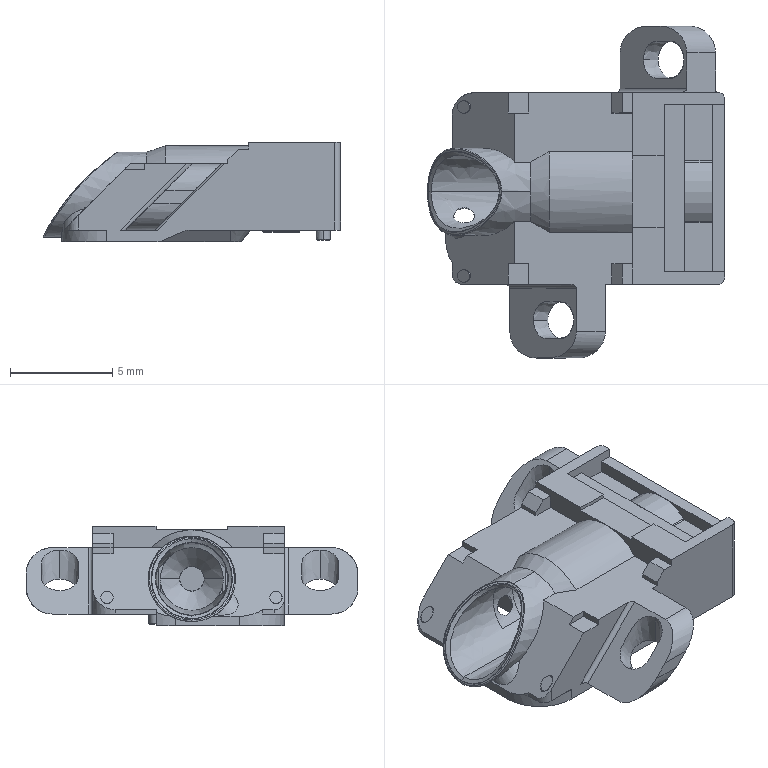Part | NX | 1 solid | 456 faces | box 14.51 x 16.208 x 4.858 mm | volume 272.047 mm3 | plane 263 | cylinder 126 | spline 25 | cone 18 | torus 18 | sphere 6 | commonest cylinder face diameters 0.2 x48 1 x17 0.4 x12 0.6 x8 0.7 x4 1.2 x4